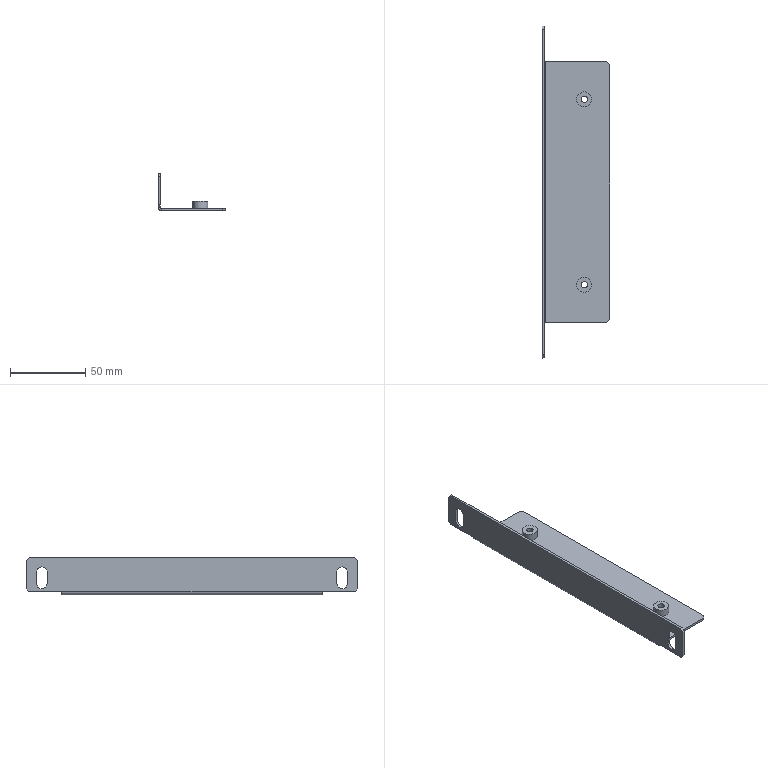Part | SolidWorks | features ICE 3, HoleWzd 2, Chamfer 1, FlatPattern 1, SMBaseFlange 1, SheetMetal 1 | 3 solids | 48 faces | box 45 x 220 x 25 mm | volume 19511 mm3 | plane 28 | cylinder 20 | commonest cylinder face diameters 7 x6 4.2 x4 5.5 x4 10 x4 1.473 x1 4.473 x1
STEP:
#1=CARTESIAN_POINT('',(25.9,61.5,-18.5));
#2=VERTEX_POINT('',#1);
#3=CARTESIAN_POINT('',(30.1,61.5,-18.5));
#4=VERTEX_POINT('',#3);
#5=CARTESIAN_POINT('',(28.,61.5,-18.5));
#6=DIRECTION('',(0.,0.,1.));
#7=DIRECTION('',(1.,0.,0.));
#8=AXIS2_PLACEMENT_3D('',#5,#6,#7);
#9=CIRCLE('',#8,2.1);
#10=EDGE_CURVE('',#2,#4,#9,.T.);
#11=ORIENTED_EDGE('',*,*,#10,.T.);
#12=CARTESIAN_POINT('',(30.1,61.5,-23.5));
#13=VERTEX_POINT('',#12);
#14=CARTESIAN_POINT('',(30.1,61.5,-23.5));
#15=DIRECTION('',(0.,0.,-1.));
#16=VECTOR('',#15,1000.);
#17=LINE('',#14,#16);
#18=EDGE_CURVE('',#4,#13,#17,.T.);
#19=ORIENTED_EDGE('',*,*,#18,.T.);
#20=CARTESIAN_POINT('',(25.9,61.5,-23.5));
#21=VERTEX_POINT('',#20);
#22=CARTESIAN_POINT('',(28.,61.5,-23.5));
#23=DIRECTION('',(0.,0.,-1.));
#24=DIRECTION('',(-1.,0.,0.));
#25=AXIS2_PLACEMENT_3D('',#22,#23,#24);
#26=CIRCLE('',#25,2.1);
#27=EDGE_CURVE('',#13,#21,#26,.T.);
#28=ORIENTED_EDGE('',*,*,#27,.T.);
#29=CARTESIAN_POINT('',(25.9,61.5,-23.5));
#30=DIRECTION('',(0.,0.,-1.));
#31=VECTOR('',#30,1000.);
#32=LINE('',#29,#31);
#33=EDGE_CURVE('',#2,#21,#32,.T.);
#34=ORIENTED_EDGE('',*,*,#33,.F.);
#35=EDGE_LOOP('',(#11,#19,#28,#34));
#36=FACE_OUTER_BOUND('',#35,.T.);
#37=CARTESIAN_POINT('',(28.,61.5,-23.5));
#38=DIRECTION('',(0.,0.,-1.));
#39=DIRECTION('',(-1.,0.,0.));
#40=AXIS2_PLACEMENT_3D('',#37,#38,#39);
#41=CYLINDRICAL_SURFACE('',#40,2.1);
#42=ADVANCED_FACE('',(#36),#41,.F.);
#43=CARTESIAN_POINT('',(33.,61.5,-18.5));
#44=VERTEX_POINT('',#43);
#45=CARTESIAN_POINT('',(23.,61.5,-18.5));
#46=VERTEX_POINT('',#45);
#47=CARTESIAN_POINT('',(28.,61.5,-18.5));
#48=DIRECTION('',(0.,0.,1.));
#49=DIRECTION('',(1.,0.,0.));
#50=AXIS2_PLACEMENT_3D('',#47,#48,#49);
#51=CIRCLE('',#50,5.);
#52=EDGE_CURVE('',#44,#46,#51,.T.);
#53=ORIENTED_EDGE('',*,*,#52,.F.);
#54=CARTESIAN_POINT('',(33.,61.5,-23.5));
#55=VERTEX_POINT('',#54);
#56=CARTESIAN_POINT('',(33.,61.5,-18.5));
#57=DIRECTION('',(0.,0.,-1.));
#58=VECTOR('',#57,1000.);
#59=LINE('',#56,#58);
#60=EDGE_CURVE('',#44,#55,#59,.T.);
#61=ORIENTED_EDGE('',*,*,#60,.T.);
#62=CARTESIAN_POINT('',(23.,61.5,-23.5));
#63=VERTEX_POINT('',#62);
#64=CARTESIAN_POINT('',(28.,61.5,-23.5));
#65=DIRECTION('',(0.,0.,1.));
#66=DIRECTION('',(1.,0.,0.));
#67=AXIS2_PLACEMENT_3D('',#64,#65,#66);
#68=CIRCLE('',#67,5.);
#69=EDGE_CURVE('',#55,#63,#68,.T.);
#70=ORIENTED_EDGE('',*,*,#69,.T.);
#71=CARTESIAN_POINT('',(23.,61.5,-18.5));
#72=DIRECTION('',(0.,0.,-1.));
#73=VECTOR('',#72,1000.);
#74=LINE('',#71,#73);
#75=EDGE_CURVE('',#46,#63,#74,.T.);
#76=ORIENTED_EDGE('',*,*,#75,.F.);
#77=EDGE_LOOP('',(#53,#61,#70,#76));
#78=FACE_OUTER_BOUND('',#77,.T.);
#79=CARTESIAN_POINT('',(28.,61.5,-18.5));
#80=DIRECTION('',(0.,0.,-1.));
#81=DIRECTION('',(-1.,0.,0.));
#82=AXIS2_PLACEMENT_3D('',#79,#80,#81);
#83=CYLINDRICAL_SURFACE('',#82,5.);
#84=ADVANCED_FACE('',(#78),#83,.T.);
#85=ORIENTED_EDGE('',*,*,#60,.F.);
#86=CARTESIAN_POINT('',(28.,61.5,-18.5));
#87=DIRECTION('',(0.,0.,1.));
#88=DIRECTION('',(1.,0.,0.));
#89=AXIS2_PLACEMENT_3D('',#86,#87,#88);
#90=CIRCLE('',#89,5.);
#91=EDGE_CURVE('',#46,#44,#90,.T.);
#92=ORIENTED_EDGE('',*,*,#91,.F.);
#93=ORIENTED_EDGE('',*,*,#75,.T.);
#94=CARTESIAN_POINT('',(28.,61.5,-23.5));
#95=DIRECTION('',(0.,0.,1.));
#96=DIRECTION('',(1.,0.,0.));
#97=AXIS2_PLACEMENT_3D('',#94,#95,#96);
#98=CIRCLE('',#97,5.);
#99=EDGE_CURVE('',#63,#55,#98,.T.);
#100=ORIENTED_EDGE('',*,*,#99,.T.);
#101=EDGE_LOOP('',(#85,#92,#93,#100));
#102=FACE_OUTER_BOUND('',#101,.T.);
#103=CARTESIAN_POINT('',(28.,61.5,-18.5));
#104=DIRECTION('',(0.,0.,-1.));
#105=DIRECTION('',(-1.,0.,0.));
#106=AXIS2_PLACEMENT_3D('',#103,#104,#105);
#107=CYLINDRICAL_SURFACE('',#106,5.);
#108=ADVANCED_FACE('',(#102),#107,.T.);
#109=ORIENTED_EDGE('',*,*,#10,.F.);
#110=CARTESIAN_POINT('',(28.,61.5,-18.5));
#111=DIRECTION('',(0.,0.,1.));
#112=DIRECTION('',(1.,0.,0.));
#113=AXIS2_PLACEMENT_3D('',#110,#111,#112);
#114=CIRCLE('',#113,2.1);
#115=EDGE_CURVE('',#4,#2,#114,.T.);
#116=ORIENTED_EDGE('',*,*,#115,.F.);
#117=EDGE_LOOP('',(#109,#116));
#118=FACE_BOUND('',#117,.T.);
#119=ORIENTED_EDGE('',*,*,#91,.T.);
#120=ORIENTED_EDGE('',*,*,#52,.T.);
#121=EDGE_LOOP('',(#119,#120));
#122=FACE_OUTER_BOUND('',#121,.T.);
#123=CARTESIAN_POINT('',(28.,61.5,-18.5));
#124=DIRECTION('',(0.,0.,1.));
#125=DIRECTION('',(1.,0.,0.));
#126=AXIS2_PLACEMENT_3D('',#123,#124,#125);
#127=PLANE('',#126);
#128=ADVANCED_FACE('',(#118,#122),#127,.T.);
#129=CARTESIAN_POINT('',(28.,61.5,-23.5));
#130=DIRECTION('',(0.,0.,-1.));
#131=DIRECTION('',(-1.,0.,0.));
#132=AXIS2_PLACEMENT_3D('',#129,#130,#131);
#133=CIRCLE('',#132,2.1);
#134=EDGE_CURVE('',#21,#13,#133,.T.);
#135=ORIENTED_EDGE('',*,*,#134,.F.);
#136=ORIENTED_EDGE('',*,*,#27,.F.);
#137=EDGE_LOOP('',(#135,#136));
#138=FACE_BOUND('',#137,.T.);
#139=ORIENTED_EDGE('',*,*,#99,.F.);
#140=ORIENTED_EDGE('',*,*,#69,.F.);
#141=EDGE_LOOP('',(#139,#140));
#142=FACE_OUTER_BOUND('',#141,.T.);
#143=CARTESIAN_POINT('',(28.,61.5,-23.5));
#144=DIRECTION('',(0.,0.,1.));
#145=DIRECTION('',(1.,0.,0.));
#146=AXIS2_PLACEMENT_3D('',#143,#144,#145);
#147=PLANE('',#146);
#148=ADVANCED_FACE('',(#138,#142),#147,.F.);
#149=ORIENTED_EDGE('',*,*,#18,.F.);
#150=ORIENTED_EDGE('',*,*,#115,.T.);
#151=ORIENTED_EDGE('',*,*,#33,.T.);
#152=ORIENTED_EDGE('',*,*,#134,.T.);
#153=EDGE_LOOP('',(#149,#150,#151,#152));
#154=FACE_OUTER_BOUND('',#153,.T.);
#155=CARTESIAN_POINT('',(28.,61.5,-23.5));
#156=DIRECTION('',(0.,0.,-1.));
#157=DIRECTION('',(-1.,0.,0.));
#158=AXIS2_PLACEMENT_3D('',#155,#156,#157);
#159=CYLINDRICAL_SURFACE('',#158,2.1);
#160=ADVANCED_FACE('',(#154),#159,.F.);
#161=CLOSED_SHELL('',(#42,#84,#108,#128,#148,#160));
#162=MANIFOLD_SOLID_BREP('',#161);
#163=CARTESIAN_POINT('',(25.9,-61.5,-18.5));
#164=VERTEX_POINT('',#163);
#165=CARTESIAN_POINT('',(30.1,-61.5,-18.5));
#166=VERTEX_POINT('',#165);
#167=CARTESIAN_POINT('',(28.,-61.5,-18.5));
#168=DIRECTION('',(0.,0.,1.));
#169=DIRECTION('',(1.,0.,0.));
#170=AXIS2_PLACEMENT_3D('',#167,#168,#169);
#171=CIRCLE('',#170,2.1);
#172=EDGE_CURVE('',#164,#166,#171,.T.);
#173=ORIENTED_EDGE('',*,*,#172,.T.);
#174=CARTESIAN_POINT('',(30.1,-61.5,-23.5));
#175=VERTEX_POINT('',#174);
#176=CARTESIAN_POINT('',(30.1,-61.5,-23.5));
#177=DIRECTION('',(0.,0.,-1.));
#178=VECTOR('',#177,1000.);
#179=LINE('',#176,#178);
#180=EDGE_CURVE('',#166,#175,#179,.T.);
#181=ORIENTED_EDGE('',*,*,#180,.T.);
#182=CARTESIAN_POINT('',(25.9,-61.5,-23.5));
#183=VERTEX_POINT('',#182);
#184=CARTESIAN_POINT('',(28.,-61.5,-23.5));
#185=DIRECTION('',(0.,0.,-1.));
#186=DIRECTION('',(-1.,0.,0.));
#187=AXIS2_PLACEMENT_3D('',#184,#185,#186);
#188=CIRCLE('',#187,2.1);
#189=EDGE_CURVE('',#175,#183,#188,.T.);
#190=ORIENTED_EDGE('',*,*,#189,.T.);
#191=CARTESIAN_POINT('',(25.9,-61.5,-23.5));
#192=DIRECTION('',(0.,0.,-1.));
#193=VECTOR('',#192,1000.);
#194=LINE('',#191,#193);
#195=EDGE_CURVE('',#164,#183,#194,.T.);
#196=ORIENTED_EDGE('',*,*,#195,.F.);
#197=EDGE_LOOP('',(#173,#181,#190,#196));
#198=FACE_OUTER_BOUND('',#197,.T.);
#199=CARTESIAN_POINT('',(28.,-61.5,-23.5));
#200=DIRECTION('',(0.,0.,-1.));
#201=DIRECTION('',(-1.,0.,0.));
#202=AXIS2_PLACEMENT_3D('',#199,#200,#201);
#203=CYLINDRICAL_SURFACE('',#202,2.1);
#204=ADVANCED_FACE('',(#198),#203,.F.);
#205=CARTESIAN_POINT('',(33.,-61.5,-18.5));
#206=VERTEX_POINT('',#205);
#207=CARTESIAN_POINT('',(23.,-61.5,-18.5));
#208=VERTEX_POINT('',#207);
#209=CARTESIAN_POINT('',(28.,-61.5,-18.5));
#210=DIRECTION('',(0.,0.,1.));
#211=DIRECTION('',(1.,0.,0.));
#212=AXIS2_PLACEMENT_3D('',#209,#210,#211);
#213=CIRCLE('',#212,5.);
#214=EDGE_CURVE('',#206,#208,#213,.T.);
#215=ORIENTED_EDGE('',*,*,#214,.F.);
#216=CARTESIAN_POINT('',(33.,-61.5,-23.5));
#217=VERTEX_POINT('',#216);
#218=CARTESIAN_POINT('',(33.,-61.5,-18.5));
#219=DIRECTION('',(0.,0.,-1.));
#220=VECTOR('',#219,1000.);
#221=LINE('',#218,#220);
#222=EDGE_CURVE('',#206,#217,#221,.T.);
#223=ORIENTED_EDGE('',*,*,#222,.T.);
#224=CARTESIAN_POINT('',(23.,-61.5,-23.5));
#225=VERTEX_POINT('',#224);
#226=CARTESIAN_POINT('',(28.,-61.5,-23.5));
#227=DIRECTION('',(0.,0.,1.));
#228=DIRECTION('',(1.,0.,0.));
#229=AXIS2_PLACEMENT_3D('',#226,#227,#228);
#230=CIRCLE('',#229,5.);
#231=EDGE_CURVE('',#217,#225,#230,.T.);
#232=ORIENTED_EDGE('',*,*,#231,.T.);
#233=CARTESIAN_POINT('',(23.,-61.5,-18.5));
#234=DIRECTION('',(0.,0.,-1.));
#235=VECTOR('',#234,1000.);
#236=LINE('',#233,#235);
#237=EDGE_CURVE('',#208,#225,#236,.T.);
#238=ORIENTED_EDGE('',*,*,#237,.F.);
#239=EDGE_LOOP('',(#215,#223,#232,#238));
#240=FACE_OUTER_BOUND('',#239,.T.);
#241=CARTESIAN_POINT('',(28.,-61.5,-18.5));
#242=DIRECTION('',(0.,0.,-1.));
#243=DIRECTION('',(-1.,0.,0.));
#244=AXIS2_PLACEMENT_3D('',#241,#242,#243);
#245=CYLINDRICAL_SURFACE('',#244,5.);
#246=ADVANCED_FACE('',(#240),#245,.T.);
#247=ORIENTED_EDGE('',*,*,#222,.F.);
#248=CARTESIAN_POINT('',(28.,-61.5,-18.5));
#249=DIRECTION('',(0.,0.,1.));
#250=DIRECTION('',(1.,0.,0.));
#251=AXIS2_PLACEMENT_3D('',#248,#249,#250);
#252=CIRCLE('',#251,5.);
#253=EDGE_CURVE('',#208,#206,#252,.T.);
#254=ORIENTED_EDGE('',*,*,#253,.F.);
#255=ORIENTED_EDGE('',*,*,#237,.T.);
#256=CARTESIAN_POINT('',(28.,-61.5,-23.5));
#257=DIRECTION('',(0.,0.,1.));
#258=DIRECTION('',(1.,0.,0.));
#259=AXIS2_PLACEMENT_3D('',#256,#257,#258);
#260=CIRCLE('',#259,5.);
#261=EDGE_CURVE('',#225,#217,#260,.T.);
#262=ORIENTED_EDGE('',*,*,#261,.T.);
#263=EDGE_LOOP('',(#247,#254,#255,#262));
#264=FACE_OUTER_BOUND('',#263,.T.);
#265=CARTESIAN_POINT('',(28.,-61.5,-18.5));
#266=DIRECTION('',(0.,0.,-1.));
#267=DIRECTION('',(-1.,0.,0.));
#268=AXIS2_PLACEMENT_3D('',#265,#266,#267);
#269=CYLINDRICAL_SURFACE('',#268,5.);
#270=ADVANCED_FACE('',(#264),#269,.T.);
#271=ORIENTED_EDGE('',*,*,#172,.F.);
#272=CARTESIAN_POINT('',(28.,-61.5,-18.5));
#273=DIRECTION('',(0.,0.,1.));
#274=DIRECTION('',(1.,0.,0.));
#275=AXIS2_PLACEMENT_3D('',#272,#273,#274);
#276=CIRCLE('',#275,2.1);
#277=EDGE_CURVE('',#166,#164,#276,.T.);
#278=ORIENTED_EDGE('',*,*,#277,.F.);
#279=EDGE_LOOP('',(#271,#278));
#280=FACE_BOUND('',#279,.T.);
#281=ORIENTED_EDGE('',*,*,#253,.T.);
#282=ORIENTED_EDGE('',*,*,#214,.T.);
#283=EDGE_LOOP('',(#281,#282));
#284=FACE_OUTER_BOUND('',#283,.T.);
#285=CARTESIAN_POINT('',(28.,-61.5,-18.5));
#286=DIRECTION('',(0.,0.,1.));
#287=DIRECTION('',(1.,0.,0.));
#288=AXIS2_PLACEMENT_3D('',#285,#286,#287);
#289=PLANE('',#288);
#290=ADVANCED_FACE('',(#280,#284),#289,.T.);
#291=CARTESIAN_POINT('',(28.,-61.5,-23.5));
#292=DIRECTION('',(0.,0.,-1.));
#293=DIRECTION('',(-1.,0.,0.));
#294=AXIS2_PLACEMENT_3D('',#291,#292,#293);
#295=CIRCLE('',#294,2.1);
#296=EDGE_CURVE('',#183,#175,#295,.T.);
#297=ORIENTED_EDGE('',*,*,#296,.F.);
#298=ORIENTED_EDGE('',*,*,#189,.F.);
#299=EDGE_LOOP('',(#297,#298));
#300=FACE_BOUND('',#299,.T.);
#301=ORIENTED_EDGE('',*,*,#261,.F.);
#302=ORIENTED_EDGE('',*,*,#231,.F.);
#303=EDGE_LOOP('',(#301,#302));
#304=FACE_OUTER_BOUND('',#303,.T.);
#305=CARTESIAN_POINT('',(28.,-61.5,-23.5));
#306=DIRECTION('',(0.,0.,1.));
#307=DIRECTION('',(1.,0.,0.));
#308=AXIS2_PLACEMENT_3D('',#305,#306,#307);
#309=PLANE('',#308);
#310=ADVANCED_FACE('',(#300,#304),#309,.F.);
#311=ORIENTED_EDGE('',*,*,#180,.F.);
#312=ORIENTED_EDGE('',*,*,#277,.T.);
#313=ORIENTED_EDGE('',*,*,#195,.T.);
#314=ORIENTED_EDGE('',*,*,#296,.T.);
#315=EDGE_LOOP('',(#311,#312,#313,#314));
#316=FACE_OUTER_BOUND('',#315,.T.);
#317=CARTESIAN_POINT('',(28.,-61.5,-23.5));
#318=DIRECTION('',(0.,0.,-1.));
#319=DIRECTION('',(-1.,0.,0.));
#320=AXIS2_PLACEMENT_3D('',#317,#318,#319);
#321=CYLINDRICAL_SURFACE('',#320,2.1);
#322=ADVANCED_FACE('',(#316),#321,.F.);
#323=CLOSED_SHELL('',(#204,#246,#270,#290,#310,#322));
#324=MANIFOLD_SOLID_BREP('',#323);
#325=CARTESIAN_POINT('',(1.5,-99.5,-6.5));
#326=VERTEX_POINT('',#325);
#327=CARTESIAN_POINT('',(1.5,-96.,-10.));
#328=VERTEX_POINT('',#327);
#329=CARTESIAN_POINT('',(1.5,-99.5,-10.));
#330=DIRECTION('',(-1.,0.,0.));
#331=DIRECTION('',(0.,0.,1.));
#332=AXIS2_PLACEMENT_3D('',#329,#330,#331);
#333=CIRCLE('',#332,3.5);
#334=EDGE_CURVE('',#326,#328,#333,.T.);
#335=ORIENTED_EDGE('',*,*,#334,.F.);
#336=CARTESIAN_POINT('',(0.,-99.5,-6.5));
#337=VERTEX_POINT('',#336);
#338=CARTESIAN_POINT('',(5.,-99.5,-6.5));
#339=DIRECTION('',(-1.,0.,0.));
#340=VECTOR('',#339,1000.);
#341=LINE('',#338,#340);
#342=EDGE_CURVE('',#326,#337,#341,.T.);
#343=ORIENTED_EDGE('',*,*,#342,.T.);
#344=CARTESIAN_POINT('',(0.,-96.,-10.));
#345=VERTEX_POINT('',#344);
#346=CARTESIAN_POINT('',(0.,-99.5,-10.));
#347=DIRECTION('',(-1.,0.,0.));
#348=DIRECTION('',(0.,0.,1.));
#349=AXIS2_PLACEMENT_3D('',#346,#347,#348);
#350=CIRCLE('',#349,3.5);
#351=EDGE_CURVE('',#337,#345,#350,.T.);
#352=ORIENTED_EDGE('',*,*,#351,.T.);
#353=CARTESIAN_POINT('',(5.,-96.,-10.));
#354=DIRECTION('',(-1.,0.,0.));
#355=VECTOR('',#354,1000.);
#356=LINE('',#353,#355);
#357=EDGE_CURVE('',#328,#345,#356,.T.);
#358=ORIENTED_EDGE('',*,*,#357,.F.);
#359=EDGE_LOOP('',(#335,#343,#352,#358));
#360=FACE_OUTER_BOUND('',#359,.T.);
#361=CARTESIAN_POINT('',(5.,-99.5,-10.));
#362=DIRECTION('',(-1.,0.,0.));
#363=DIRECTION('',(0.,0.,1.));
#364=AXIS2_PLACEMENT_3D('',#361,#362,#363);
#365=CYLINDRICAL_SURFACE('',#364,3.5);
#366=ADVANCED_FACE('',(#360),#365,.F.);
#367=CARTESIAN_POINT('',(1.5,99.5,-6.5));
#368=VERTEX_POINT('',#367);
#369=CARTESIAN_POINT('',(1.5,103.,-10.));
#370=VERTEX_POINT('',#369);
#371=CARTESIAN_POINT('',(1.5,99.5,-10.));
#372=DIRECTION('',(-1.,0.,0.));
#373=DIRECTION('',(0.,0.,1.));
#374=AXIS2_PLACEMENT_3D('',#371,#372,#373);
#375=CIRCLE('',#374,3.5);
#376=EDGE_CURVE('',#368,#370,#375,.T.);
#377=ORIENTED_EDGE('',*,*,#376,.F.);
#378=CARTESIAN_POINT('',(0.,99.5,-6.5));
#379=VERTEX_POINT('',#378);
#380=CARTESIAN_POINT('',(5.,99.5,-6.5));
#381=DIRECTION('',(-1.,0.,0.));
#382=VECTOR('',#381,1000.);
#383=LINE('',#380,#382);
#384=EDGE_CURVE('',#368,#379,#383,.T.);
#385=ORIENTED_EDGE('',*,*,#384,.T.);
#386=CARTESIAN_POINT('',(0.,103.,-10.));
#387=VERTEX_POINT('',#386);
#388=CARTESIAN_POINT('',(0.,99.5,-10.));
#389=DIRECTION('',(-1.,0.,0.));
#390=DIRECTION('',(0.,0.,1.));
#391=AXIS2_PLACEMENT_3D('',#388,#389,#390);
#392=CIRCLE('',#391,3.5);
#393=EDGE_CURVE('',#379,#387,#392,.T.);
#394=ORIENTED_EDGE('',*,*,#393,.T.);
#395=CARTESIAN_POINT('',(5.,103.,-10.));
#396=DIRECTION('',(-1.,0.,0.));
#397=VECTOR('',#396,1000.);
#398=LINE('',#395,#397);
#399=EDGE_CURVE('',#370,#387,#398,.T.);
#400=ORIENTED_EDGE('',*,*,#399,.F.);
#401=EDGE_LOOP('',(#377,#385,#394,#400));
#402=FACE_OUTER_BOUND('',#401,.T.);
#403=CARTESIAN_POINT('',(5.,99.5,-10.));
#404=DIRECTION('',(-1.,0.,0.));
#405=DIRECTION('',(0.,0.,1.));
#406=AXIS2_PLACEMENT_3D('',#403,#404,#405);
#407=CYLINDRICAL_SURFACE('',#406,3.5);
#408=ADVANCED_FACE('',(#402),#407,.F.);
#409=CARTESIAN_POINT('',(30.75,61.5,-23.5));
#410=VERTEX_POINT('',#409);
#411=CARTESIAN_POINT('',(25.25,61.5,-23.5));
#412=VERTEX_POINT('',#411);
#413=CARTESIAN_POINT('',(28.,61.5,-23.5));
#414=DIRECTION('',(0.,0.,-1.));
#415=DIRECTION('',(-1.,0.,0.));
#416=AXIS2_PLACEMENT_3D('',#413,#414,#415);
#417=CIRCLE('',#416,2.75);
#418=EDGE_CURVE('',#410,#412,#417,.T.);
#419=ORIENTED_EDGE('',*,*,#418,.F.);
#420=CARTESIAN_POINT('',(30.75,61.5,-25.));
#421=VERTEX_POINT('',#420);
#422=CARTESIAN_POINT('',(30.75,61.5,-25.));
#423=DIRECTION('',(0.,0.,-1.));
#424=VECTOR('',#423,1000.);
#425=LINE('',#422,#424);
#426=EDGE_CURVE('',#410,#421,#425,.T.);
#427=ORIENTED_EDGE('',*,*,#426,.T.);
#428=CARTESIAN_POINT('',(25.25,61.5,-25.));
#429=VERTEX_POINT('',#428);
#430=CARTESIAN_POINT('',(28.,61.5,-25.));
#431=DIRECTION('',(0.,0.,-1.));
#432=DIRECTION('',(-1.,0.,0.));
#433=AXIS2_PLACEMENT_3D('',#430,#431,#432);
#434=CIRCLE('',#433,2.75);
#435=EDGE_CURVE('',#421,#429,#434,.T.);
#436=ORIENTED_EDGE('',*,*,#435,.T.);
#437=CARTESIAN_POINT('',(25.25,61.5,-25.));
#438=DIRECTION('',(0.,0.,-1.));
#439=VECTOR('',#438,1000.);
#440=LINE('',#437,#439);
#441=EDGE_CURVE('',#412,#429,#440,.T.);
#442=ORIENTED_EDGE('',*,*,#441,.F.);
#443=EDGE_LOOP('',(#419,#427,#436,#442));
#444=FACE_OUTER_BOUND('',#443,.T.);
#445=CARTESIAN_POINT('',(28.,61.5,-25.));
#446=DIRECTION('',(0.,0.,-1.));
#447=DIRECTION('',(-1.,0.,0.));
#448=AXIS2_PLACEMENT_3D('',#445,#446,#447);
#449=CYLINDRICAL_SURFACE('',#448,2.75);
#450=ADVANCED_FACE('',(#444),#449,.F.);
#451=CARTESIAN_POINT('',(30.75,-61.5,-23.5));
#452=VERTEX_POINT('',#451);
#453=CARTESIAN_POINT('',(25.25,-61.5,-23.5));
#454=VERTEX_POINT('',#453);
#455=CARTESIAN_POINT('',(28.,-61.5,-23.5));
#456=DIRECTION('',(0.,0.,-1.));
#457=DIRECTION('',(-1.,0.,0.));
#458=AXIS2_PLACEMENT_3D('',#455,#456,#457);
#459=CIRCLE('',#458,2.75);
#460=EDGE_CURVE('',#452,#454,#459,.T.);
#461=ORIENTED_EDGE('',*,*,#460,.F.);
#462=CARTESIAN_POINT('',(30.75,-61.5,-25.));
#463=VERTEX_POINT('',#462);
#464=CARTESIAN_POINT('',(30.75,-61.5,-25.));
#465=DIRECTION('',(0.,0.,-1.));
#466=VECTOR('',#465,1000.);
#467=LINE('',#464,#466);
#468=EDGE_CURVE('',#452,#463,#467,.T.);
#469=ORIENTED_EDGE('',*,*,#468,.T.);
#470=CARTESIAN_POINT('',(25.25,-61.5,-25.));
#471=VERTEX_POINT('',#470);
#472=CARTESIAN_POINT('',(28.,-61.5,-25.));
#473=DIRECTION('',(0.,0.,-1.));
#474=DIRECTION('',(-1.,0.,0.));
#475=AXIS2_PLACEMENT_3D('',#472,#473,#474);
#476=CIRCLE('',#475,2.75);
#477=EDGE_CURVE('',#463,#471,#476,.T.);
#478=ORIENTED_EDGE('',*,*,#477,.T.);
#479=CARTESIAN_POINT('',(25.25,-61.5,-25.));
#480=DIRECTION('',(0.,0.,-1.));
#481=VECTOR('',#480,1000.);
#482=LINE('',#479,#481);
#483=EDGE_CURVE('',#454,#471,#482,.T.);
#484=ORIENTED_EDGE('',*,*,#483,.F.);
#485=EDGE_LOOP('',(#461,#469,#478,#484));
#486=FACE_OUTER_BOUND('',#485,.T.);
#487=CARTESIAN_POINT('',(28.,-61.5,-25.));
#488=DIRECTION('',(0.,0.,-1.));
#489=DIRECTION('',(-1.,0.,0.));
#490=AXIS2_PLACEMENT_3D('',#487,#488,#489);
#491=CYLINDRICAL_SURFACE('',#490,2.75);
#492=ADVANCED_FACE('',(#486),#491,.F.);
#493=CARTESIAN_POINT('',(28.,61.5,-23.5));
#494=DIRECTION('',(0.,0.,-1.));
#495=DIRECTION('',(-1.,0.,0.));
#496=AXIS2_PLACEMENT_3D('',#493,#494,#495);
#497=CIRCLE('',#496,2.75);
#498=EDGE_CURVE('',#412,#410,#497,.T.);
#499=ORIENTED_EDGE('',*,*,#498,.T.);
#500=ORIENTED_EDGE('',*,*,#418,.T.);
#501=EDGE_LOOP('',(#499,#500));
#502=FACE_BOUND('',#501,.T.);
#503=CARTESIAN_POINT('',(28.,-61.5,-23.5));
#504=DIRECTION('',(0.,0.,-1.));
#505=DIRECTION('',(-1.,0.,0.));
#506=AXIS2_PLACEMENT_3D('',#503,#504,#505);
#507=CIRCLE('',#506,2.75);
#508=EDGE_CURVE('',#454,#452,#507,.T.);
#509=ORIENTED_EDGE('',*,*,#508,.T.);
#510=ORIENTED_EDGE('',*,*,#460,.T.);
#511=EDGE_LOOP('',(#509,#510));
#512=FACE_BOUND('',#511,.T.);
#513=CARTESIAN_POINT('',(2.237,-86.5,-23.5));
#514=VERTEX_POINT('',#513);
#515=CARTESIAN_POINT('',(43.,-86.5,-23.5));
#516=VERTEX_POINT('',#515);
#517=CARTESIAN_POINT('',(0.,-86.5,-23.5));
#518=DIRECTION('',(1.,0.,0.));
#519=VECTOR('',#518,1000.);
#520=LINE('',#517,#519);
#521=EDGE_CURVE('',#514,#516,#520,.T.);
#522=ORIENTED_EDGE('',*,*,#521,.T.);
#523=CARTESIAN_POINT('',(45.,-84.5,-23.5));
#524=VERTEX_POINT('',#523);
#525=CARTESIAN_POINT('',(45.,-84.5,-23.5));
#526=DIRECTION('',(0.7071,0.7071,0.));
#527=VECTOR('',#526,1000.);
#528=LINE('',#525,#527);
#529=EDGE_CURVE('',#516,#524,#528,.T.);
#530=ORIENTED_EDGE('',*,*,#529,.T.);
#531=CARTESIAN_POINT('',(45.,84.5,-23.5));
#532=VERTEX_POINT('',#531);
#533=CARTESIAN_POINT('',(45.,110.,-23.5));
#534=DIRECTION('',(0.,-1.,0.));
#535=VECTOR('',#534,1000.);
#536=LINE('',#533,#535);
#537=EDGE_CURVE('',#532,#524,#536,.T.);
#538=ORIENTED_EDGE('',*,*,#537,.F.);
#539=CARTESIAN_POINT('',(43.,86.5,-23.5));
#540=VERTEX_POINT('',#539);
#541=CARTESIAN_POINT('',(45.,84.5,-23.5));
#542=DIRECTION('',(-0.7071,0.7071,0.));
#543=VECTOR('',#542,1000.);
#544=LINE('',#541,#543);
#545=EDGE_CURVE('',#532,#540,#544,.T.);
#546=ORIENTED_EDGE('',*,*,#545,.T.);
#547=CARTESIAN_POINT('',(2.237,86.5,-23.5));
#548=VERTEX_POINT('',#547);
#549=CARTESIAN_POINT('',(0.,86.5,-23.5));
#550=DIRECTION('',(-1.,0.,0.));
#551=VECTOR('',#550,1000.);
#552=LINE('',#549,#551);
#553=EDGE_CURVE('',#540,#548,#552,.T.);
#554=ORIENTED_EDGE('',*,*,#553,.T.);
#555=CARTESIAN_POINT('',(2.237,110.,-23.5));
#556=DIRECTION('',(0.,-1.,0.));
#557=VECTOR('',#556,1000.);
#558=LINE('',#555,#557);
#559=EDGE_CURVE('',#548,#514,#558,.T.);
#560=ORIENTED_EDGE('',*,*,#559,.T.);
#561=EDGE_LOOP('',(#522,#530,#538,#546,#554,#560));
#562=FACE_OUTER_BOUND('',#561,.T.);
#563=CARTESIAN_POINT('',(0.,110.,-23.5));
#564=DIRECTION('',(0.,0.,-1.));
#565=DIRECTION('',(-1.,0.,0.));
#566=AXIS2_PLACEMENT_3D('',#563,#564,#565);
#567=PLANE('',#566);
#568=ADVANCED_FACE('',(#502,#512,#562),#567,.F.);
#569=ORIENTED_EDGE('',*,*,#537,.T.);
#570=CARTESIAN_POINT('',(45.,-84.5,-25.));
#571=VERTEX_POINT('',#570);
#572=CARTESIAN_POINT('',(45.,-84.5,-25.));
#573=DIRECTION('',(0.,0.,-1.));
#574=VECTOR('',#573,1000.);
#575=LINE('',#572,#574);
#576=EDGE_CURVE('',#524,#571,#575,.T.);
#577=ORIENTED_EDGE('',*,*,#576,.T.);
#578=CARTESIAN_POINT('',(45.,84.5,-25.));
#579=VERTEX_POINT('',#578);
#580=CARTESIAN_POINT('',(45.,110.,-25.));
#581=DIRECTION('',(0.,-1.,0.));
#582=VECTOR('',#581,1000.);
#583=LINE('',#580,#582);
#584=EDGE_CURVE('',#579,#571,#583,.T.);
#585=ORIENTED_EDGE('',*,*,#584,.F.);
#586=CARTESIAN_POINT('',(45.,84.5,-25.));
#587=DIRECTION('',(0.,0.,1.));
#588=VECTOR('',#587,1000.);
#589=LINE('',#586,#588);
#590=EDGE_CURVE('',#579,#532,#589,.T.);
#591=ORIENTED_EDGE('',*,*,#590,.T.);
#592=EDGE_LOOP('',(#569,#577,#585,#591));
#593=FACE_OUTER_BOUND('',#592,.T.);
#594=CARTESIAN_POINT('',(45.,110.,-25.));
#595=DIRECTION('',(1.,0.,0.));
#596=DIRECTION('',(0.,0.,-1.));
#597=AXIS2_PLACEMENT_3D('',#594,#595,#596);
#598=PLANE('',#597);
#599=ADVANCED_FACE('',(#593),#598,.T.);
#600=CARTESIAN_POINT('',(28.,61.5,-25.));
#601=DIRECTION('',(0.,0.,-1.));
#602=DIRECTION('',(-1.,0.,0.));
#603=AXIS2_PLACEMENT_3D('',#600,#601,#602);
#604=CIRCLE('',#603,2.75);
#605=EDGE_CURVE('',#429,#421,#604,.T.);
#606=ORIENTED_EDGE('',*,*,#605,.F.);
#607=ORIENTED_EDGE('',*,*,#435,.F.);
#608=EDGE_LOOP('',(#606,#607));
#609=FACE_BOUND('',#608,.T.);
#610=CARTESIAN_POINT('',(28.,-61.5,-25.));
#611=DIRECTION('',(0.,0.,-1.));
#612=DIRECTION('',(-1.,0.,0.));
#613=AXIS2_PLACEMENT_3D('',#610,#611,#612);
#614=CIRCLE('',#613,2.75);
#615=EDGE_CURVE('',#471,#463,#614,.T.);
#616=ORIENTED_EDGE('',*,*,#615,.F.);
#617=ORIENTED_EDGE('',*,*,#477,.F.);
#618=EDGE_LOOP('',(#616,#617));
#619=FACE_BOUND('',#618,.T.);
#620=ORIENTED_EDGE('',*,*,#584,.T.);
#621=CARTESIAN_POINT('',(43.,-86.5,-25.));
#622=VERTEX_POINT('',#621);
#623=CARTESIAN_POINT('',(119.75,-9.75,-25.));
#624=DIRECTION('',(-0.7071,-0.7071,0.));
#625=VECTOR('',#624,1000.);
#626=LINE('',#623,#625);
#627=EDGE_CURVE('',#571,#622,#626,.T.);
#628=ORIENTED_EDGE('',*,*,#627,.T.);
#629=CARTESIAN_POINT('',(2.237,-86.5,-25.));
#630=VERTEX_POINT('',#629);
#631=CARTESIAN_POINT('',(0.,-86.5,-25.));
#632=DIRECTION('',(1.,0.,0.));
#633=VECTOR('',#632,1000.);
#634=LINE('',#631,#633);
#635=EDGE_CURVE('',#630,#622,#634,.T.);
#636=ORIENTED_EDGE('',*,*,#635,.F.);
#637=CARTESIAN_POINT('',(2.237,86.5,-25.));
#638=VERTEX_POINT('',#637);
#639=CARTESIAN_POINT('',(2.237,110.,-25.));
#640=DIRECTION('',(0.,-1.,0.));
#641=VECTOR('',#640,1000.);
#642=LINE('',#639,#641);
#643=EDGE_CURVE('',#638,#630,#642,.T.);
#644=ORIENTED_EDGE('',*,*,#643,.F.);
#645=CARTESIAN_POINT('',(43.,86.5,-25.));
#646=VERTEX_POINT('',#645);
#647=CARTESIAN_POINT('',(45.,86.5,-25.));
#648=DIRECTION('',(-1.,0.,0.));
#649=VECTOR('',#648,1000.);
#650=LINE('',#647,#649);
#651=EDGE_CURVE('',#646,#638,#650,.T.);
#652=ORIENTED_EDGE('',*,*,#651,.F.);
#653=CARTESIAN_POINT('',(9.75,119.75,-25.));
#654=DIRECTION('',(0.7071,-0.7071,0.));
#655=VECTOR('',#654,1000.);
#656=LINE('',#653,#655);
#657=EDGE_CURVE('',#646,#579,#656,.T.);
#658=ORIENTED_EDGE('',*,*,#657,.T.);
#659=EDGE_LOOP('',(#620,#628,#636,#644,#652,#658));
#660=FACE_OUTER_BOUND('',#659,.T.);
#661=CARTESIAN_POINT('',(0.,110.,-25.));
#662=DIRECTION('',(0.,0.,-1.));
#663=DIRECTION('',(-1.,0.,0.));
#664=AXIS2_PLACEMENT_3D('',#661,#662,#663);
#665=PLANE('',#664);
#666=ADVANCED_FACE('',(#609,#619,#660),#665,.T.);
#667=CARTESIAN_POINT('',(0.,108.237,-22.763));
#668=VERTEX_POINT('',#667);
#669=CARTESIAN_POINT('',(0.,-108.237,-22.763));
#670=VERTEX_POINT('',#669);
#671=CARTESIAN_POINT('',(0.,110.,-22.763));
#672=DIRECTION('',(0.,-1.,0.));
#673=VECTOR('',#672,1000.);
#674=LINE('',#671,#673);
#675=EDGE_CURVE('',#668,#670,#674,.T.);
#676=ORIENTED_EDGE('',*,*,#675,.F.);
#677=CARTESIAN_POINT('',(0.01255,108.,-23.));
#678=VERTEX_POINT('',#677);
#679=CARTESIAN_POINT('',(0.,108.237,-22.763));
#680=CARTESIAN_POINT('',(0.,108.158,-22.842));
#681=CARTESIAN_POINT('',(0.004187,108.079,-22.921));
#682=CARTESIAN_POINT('',(0.01255,108.,-23.));
#683=(BOUNDED_CURVE()B_SPLINE_CURVE(3,(#679,#680,#681,#682),.UNSPECIFIED.,.F.,.F.)B_SPLINE_CURVE_WITH_KNOTS((4,4),(4.606,4.712),.UNSPECIFIED.)CURVE()GEOMETRIC_REPRESENTATION_ITEM()RATIONAL_B_SPLINE_CURVE((1.,0.9991,0.9991,1.))REPRESENTATION_ITEM(''));
#684=EDGE_CURVE('',#668,#678,#683,.T.);
#685=ORIENTED_EDGE('',*,*,#684,.T.);
#686=CARTESIAN_POINT('',(0.01255,86.5,-23.));
#687=VERTEX_POINT('',#686);
#688=CARTESIAN_POINT('',(0.01255,110.,-23.));
#689=DIRECTION('',(0.,-1.,0.));
#690=VECTOR('',#689,1000.);
#691=LINE('',#688,#690);
#692=EDGE_CURVE('',#678,#687,#691,.T.);
#693=ORIENTED_EDGE('',*,*,#692,.T.);
#694=CARTESIAN_POINT('',(2.237,86.5,-22.763));
#695=DIRECTION('',(0.,1.,0.));
#696=DIRECTION('',(1.,0.,0.));
#697=AXIS2_PLACEMENT_3D('',#694,#695,#696);
#698=CIRCLE('',#697,2.237);
#699=EDGE_CURVE('',#638,#687,#698,.T.);
#700=ORIENTED_EDGE('',*,*,#699,.F.);
#701=ORIENTED_EDGE('',*,*,#643,.T.);
#702=CARTESIAN_POINT('',(0.01255,-86.5,-23.));
#703=VERTEX_POINT('',#702);
#704=CARTESIAN_POINT('',(2.237,-86.5,-22.763));
#705=DIRECTION('',(0.,-1.,0.));
#706=DIRECTION('',(-1.,0.,0.));
#707=AXIS2_PLACEMENT_3D('',#704,#705,#706);
#708=CIRCLE('',#707,2.237);
#709=EDGE_CURVE('',#703,#630,#708,.T.);
#710=ORIENTED_EDGE('',*,*,#709,.F.);
#711=CARTESIAN_POINT('',(0.01255,-108.,-23.));
#712=VERTEX_POINT('',#711);
#713=CARTESIAN_POINT('',(0.01255,110.,-23.));
#714=DIRECTION('',(0.,1.,0.));
#715=VECTOR('',#714,1000.);
#716=LINE('',#713,#715);
#717=EDGE_CURVE('',#712,#703,#716,.T.);
#718=ORIENTED_EDGE('',*,*,#717,.F.);
#719=CARTESIAN_POINT('',(0.01255,-108.,-23.));
#720=CARTESIAN_POINT('',(0.004187,-108.079,-22.921));
#721=CARTESIAN_POINT('',(0.,-108.158,-22.842));
#722=CARTESIAN_POINT('',(0.,-108.237,-22.763));
#723=(BOUNDED_CURVE()B_SPLINE_CURVE(3,(#719,#720,#721,#722),.UNSPECIFIED.,.F.,.F.)B_SPLINE_CURVE_WITH_KNOTS((4,4),(4.712,4.818),.UNSPECIFIED.)CURVE()GEOMETRIC_REPRESENTATION_ITEM()RATIONAL_B_SPLINE_CURVE((1.,0.9991,0.9991,1.))REPRESENTATION_ITEM(''));
#724=EDGE_CURVE('',#712,#670,#723,.T.);
#725=ORIENTED_EDGE('',*,*,#724,.T.);
#726=EDGE_LOOP('',(#676,#685,#693,#700,#701,#710,#718,#725));
#727=FACE_OUTER_BOUND('',#726,.T.);
#728=CARTESIAN_POINT('',(2.237,110.,-22.763));
#729=DIRECTION('',(0.,-1.,0.));
#730=DIRECTION('',(0.,0.,-1.));
#731=AXIS2_PLACEMENT_3D('',#728,#729,#730);
#732=CYLINDRICAL_SURFACE('',#731,2.237);
#733=ADVANCED_FACE('',(#727),#732,.T.);
#734=CARTESIAN_POINT('',(1.504,108.,-22.841));
#735=VERTEX_POINT('',#734);
#736=CARTESIAN_POINT('',(1.504,86.5,-22.841));
#737=VERTEX_POINT('',#736);
#738=CARTESIAN_POINT('',(1.504,110.,-22.841));
#739=DIRECTION('',(0.,-1.,0.));
#740=VECTOR('',#739,1000.);
#741=LINE('',#738,#740);
#742=EDGE_CURVE('',#735,#737,#741,.T.);
#743=ORIENTED_EDGE('',*,*,#742,.F.);
#744=CARTESIAN_POINT('',(1.5,108.078,-22.763));
#745=VERTEX_POINT('',#744);
#746=CARTESIAN_POINT('',(1.504,108.,-22.841));
#747=CARTESIAN_POINT('',(1.501,108.026,-22.815));
#748=CARTESIAN_POINT('',(1.5,108.052,-22.789));
#749=CARTESIAN_POINT('',(1.5,108.078,-22.763));
#750=(BOUNDED_CURVE()B_SPLINE_CURVE(3,(#746,#747,#748,#749),.UNSPECIFIED.,.F.,.F.)B_SPLINE_CURVE_WITH_KNOTS((4,4),(1.571,1.677),.UNSPECIFIED.)CURVE()GEOMETRIC_REPRESENTATION_ITEM()RATIONAL_B_SPLINE_CURVE((1.,0.9991,0.9991,1.))REPRESENTATION_ITEM(''));
#751=EDGE_CURVE('',#735,#745,#750,.T.);
#752=ORIENTED_EDGE('',*,*,#751,.T.);
#753=CARTESIAN_POINT('',(1.5,-108.078,-22.763));
#754=VERTEX_POINT('',#753);
#755=CARTESIAN_POINT('',(1.5,110.,-22.763));
#756=DIRECTION('',(0.,-1.,0.));
#757=VECTOR('',#756,1000.);
#758=LINE('',#755,#757);
#759=EDGE_CURVE('',#745,#754,#758,.T.);
#760=ORIENTED_EDGE('',*,*,#759,.T.);
#761=CARTESIAN_POINT('',(1.504,-108.,-22.841));
#762=VERTEX_POINT('',#761);
#763=CARTESIAN_POINT('',(1.5,-108.078,-22.763));
#764=CARTESIAN_POINT('',(1.5,-108.052,-22.789));
#765=CARTESIAN_POINT('',(1.501,-108.026,-22.815));
#766=CARTESIAN_POINT('',(1.504,-108.,-22.841));
#767=(BOUNDED_CURVE()B_SPLINE_CURVE(3,(#763,#764,#765,#766),.UNSPECIFIED.,.F.,.F.)B_SPLINE_CURVE_WITH_KNOTS((4,4),(1.465,1.571),.UNSPECIFIED.)CURVE()GEOMETRIC_REPRESENTATION_ITEM()RATIONAL_B_SPLINE_CURVE((1.,0.9991,0.9991,1.))REPRESENTATION_ITEM(''));
#768=EDGE_CURVE('',#754,#762,#767,.T.);
#769=ORIENTED_EDGE('',*,*,#768,.T.);
#770=CARTESIAN_POINT('',(1.504,-86.5,-22.841));
#771=VERTEX_POINT('',#770);
#772=CARTESIAN_POINT('',(1.504,110.,-22.841));
#773=DIRECTION('',(0.,1.,0.));
#774=VECTOR('',#773,1000.);
#775=LINE('',#772,#774);
#776=EDGE_CURVE('',#762,#771,#775,.T.);
#777=ORIENTED_EDGE('',*,*,#776,.T.);
#778=CARTESIAN_POINT('',(2.237,-86.5,-22.763));
#779=DIRECTION('',(0.,-1.,0.));
#780=DIRECTION('',(0.,0.,-1.));
#781=AXIS2_PLACEMENT_3D('',#778,#779,#780);
#782=CIRCLE('',#781,0.7366);
#783=EDGE_CURVE('',#771,#514,#782,.T.);
#784=ORIENTED_EDGE('',*,*,#783,.T.);
#785=ORIENTED_EDGE('',*,*,#559,.F.);
#786=CARTESIAN_POINT('',(2.237,86.5,-22.763));
#787=DIRECTION('',(0.,1.,0.));
#788=DIRECTION('',(0.,0.,-1.));
#789=AXIS2_PLACEMENT_3D('',#786,#787,#788);
#790=CIRCLE('',#789,0.7366);
#791=EDGE_CURVE('',#548,#737,#790,.T.);
#792=ORIENTED_EDGE('',*,*,#791,.T.);
#793=EDGE_LOOP('',(#743,#752,#760,#769,#777,#784,#785,#792));
#794=FACE_OUTER_BOUND('',#793,.T.);
#795=CARTESIAN_POINT('',(2.237,110.,-22.763));
#796=DIRECTION('',(0.,-1.,0.));
#797=DIRECTION('',(0.,0.,-1.));
#798=AXIS2_PLACEMENT_3D('',#795,#796,#797);
#799=CYLINDRICAL_SURFACE('',#798,0.7366);
#800=ADVANCED_FACE('',(#794),#799,.F.);
#801=CARTESIAN_POINT('',(1.5,-110.,-2.));
#802=VERTEX_POINT('',#801);
#803=CARTESIAN_POINT('',(1.5,-110.,-20.83));
#804=VERTEX_POINT('',#803);
#805=CARTESIAN_POINT('',(1.5,-110.,0.));
#806=DIRECTION('',(0.,0.,-1.));
#807=VECTOR('',#806,1000.);
#808=LINE('',#805,#807);
#809=EDGE_CURVE('',#802,#804,#808,.T.);
#810=ORIENTED_EDGE('',*,*,#809,.F.);
#811=CARTESIAN_POINT('',(0.,-110.,-2.));
#812=VERTEX_POINT('',#811);
#813=CARTESIAN_POINT('',(2.237,-110.,-2.));
#814=DIRECTION('',(-1.,0.,0.));
#815=VECTOR('',#814,1000.);
#816=LINE('',#813,#815);
#817=EDGE_CURVE('',#802,#812,#816,.T.);
#818=ORIENTED_EDGE('',*,*,#817,.T.);
#819=CARTESIAN_POINT('',(0.,-110.,-20.99));
#820=VERTEX_POINT('',#819);
#821=CARTESIAN_POINT('',(0.,-110.,0.));
#822=DIRECTION('',(0.,0.,-1.));
#823=VECTOR('',#822,1000.);
#824=LINE('',#821,#823);
#825=EDGE_CURVE('',#812,#820,#824,.T.);
#826=ORIENTED_EDGE('',*,*,#825,.T.);
#827=CARTESIAN_POINT('',(1.948,-110.,-20.783));
#828=DIRECTION('',(0.9944,0.,0.1058));
#829=VECTOR('',#828,1000.);
#830=LINE('',#827,#829);
#831=EDGE_CURVE('',#820,#804,#830,.T.);
#832=ORIENTED_EDGE('',*,*,#831,.T.);
#833=EDGE_LOOP('',(#810,#818,#826,#832));
#834=FACE_OUTER_BOUND('',#833,.T.);
#835=CARTESIAN_POINT('',(2.237,-110.,-23.5));
#836=DIRECTION('',(0.,-1.,0.));
#837=DIRECTION('',(0.,0.,-1.));
#838=AXIS2_PLACEMENT_3D('',#835,#836,#837);
#839=PLANE('',#838);
#840=ADVANCED_FACE('',(#834),#839,.T.);
#841=CARTESIAN_POINT('',(0.,-96.,-17.5));
#842=VERTEX_POINT('',#841);
#843=CARTESIAN_POINT('',(0.,-103.,-17.5));
#844=VERTEX_POINT('',#843);
#845=CARTESIAN_POINT('',(0.,-99.5,-17.5));
#846=DIRECTION('',(-1.,0.,0.));
#847=DIRECTION('',(0.,0.,1.));
#848=AXIS2_PLACEMENT_3D('',#845,#846,#847);
#849=CIRCLE('',#848,3.5);
#850=EDGE_CURVE('',#842,#844,#849,.T.);
#851=ORIENTED_EDGE('',*,*,#850,.F.);
#852=CARTESIAN_POINT('',(0.,-96.,-17.5));
#853=DIRECTION('',(0.,0.,-1.));
#854=VECTOR('',#853,1000.);
#855=LINE('',#852,#854);
#856=EDGE_CURVE('',#345,#842,#855,.T.);
#857=ORIENTED_EDGE('',*,*,#856,.F.);
#858=ORIENTED_EDGE('',*,*,#351,.F.);
#859=CARTESIAN_POINT('',(0.,-103.,-10.));
#860=VERTEX_POINT('',#859);
#861=CARTESIAN_POINT('',(0.,-99.5,-10.));
#862=DIRECTION('',(-1.,0.,0.));
#863=DIRECTION('',(0.,0.,1.));
#864=AXIS2_PLACEMENT_3D('',#861,#862,#863);
#865=CIRCLE('',#864,3.5);
#866=EDGE_CURVE('',#860,#337,#865,.T.);
#867=ORIENTED_EDGE('',*,*,#866,.F.);
#868=CARTESIAN_POINT('',(0.,-103.,-17.5));
#869=DIRECTION('',(0.,0.,1.));
#870=VECTOR('',#869,1000.);
#871=LINE('',#868,#870);
#872=EDGE_CURVE('',#844,#860,#871,.T.);
#873=ORIENTED_EDGE('',*,*,#872,.F.);
#874=EDGE_LOOP('',(#851,#857,#858,#867,#873));
#875=FACE_BOUND('',#874,.T.);
#876=CARTESIAN_POINT('',(0.,103.,-17.5));
#877=VERTEX_POINT('',#876);
#878=CARTESIAN_POINT('',(0.,96.,-17.5));
#879=VERTEX_POINT('',#878);
#880=CARTESIAN_POINT('',(0.,99.5,-17.5));
#881=DIRECTION('',(-1.,0.,0.));
#882=DIRECTION('',(0.,0.,1.));
#883=AXIS2_PLACEMENT_3D('',#880,#881,#882);
#884=CIRCLE('',#883,3.5);
#885=EDGE_CURVE('',#877,#879,#884,.T.);
#886=ORIENTED_EDGE('',*,*,#885,.F.);
#887=CARTESIAN_POINT('',(0.,103.,-17.5));
#888=DIRECTION('',(0.,0.,-1.));
#889=VECTOR('',#888,1000.);
#890=LINE('',#887,#889);
#891=EDGE_CURVE('',#387,#877,#890,.T.);
#892=ORIENTED_EDGE('',*,*,#891,.F.);
#893=ORIENTED_EDGE('',*,*,#393,.F.);
#894=CARTESIAN_POINT('',(0.,96.,-10.));
#895=VERTEX_POINT('',#894);
#896=CARTESIAN_POINT('',(0.,99.5,-10.));
#897=DIRECTION('',(-1.,0.,0.));
#898=DIRECTION('',(0.,0.,1.));
#899=AXIS2_PLACEMENT_3D('',#896,#897,#898);
#900=CIRCLE('',#899,3.5);
#901=EDGE_CURVE('',#895,#379,#900,.T.);
#902=ORIENTED_EDGE('',*,*,#901,.F.);
#903=CARTESIAN_POINT('',(0.,96.,-17.5));
#904=DIRECTION('',(0.,0.,1.));
#905=VECTOR('',#904,1000.);
#906=LINE('',#903,#905);
#907=EDGE_CURVE('',#879,#895,#906,.T.);
#908=ORIENTED_EDGE('',*,*,#907,.F.);
#909=EDGE_LOOP('',(#886,#892,#893,#902,#908));
#910=FACE_BOUND('',#909,.T.);
#911=CARTESIAN_POINT('',(0.,108.,0.));
#912=VERTEX_POINT('',#911);
#913=CARTESIAN_POINT('',(0.,-108.,0.));
#914=VERTEX_POINT('',#913);
#915=CARTESIAN_POINT('',(0.,110.,0.));
#916=DIRECTION('',(0.,-1.,0.));
#917=VECTOR('',#916,1000.);
#918=LINE('',#915,#917);
#919=EDGE_CURVE('',#912,#914,#918,.T.);
#920=ORIENTED_EDGE('',*,*,#919,.F.);
#921=CARTESIAN_POINT('',(0.,110.,-2.));
#922=VERTEX_POINT('',#921);
#923=CARTESIAN_POINT('',(0.,109.,-1.));
#924=DIRECTION('',(0.,0.7071,-0.7071));
#925=VECTOR('',#924,1000.);
#926=LINE('',#923,#925);
#927=EDGE_CURVE('',#912,#922,#926,.T.);
#928=ORIENTED_EDGE('',*,*,#927,.T.);
#929=CARTESIAN_POINT('',(0.,110.,-20.99));
#930=VERTEX_POINT('',#929);
#931=CARTESIAN_POINT('',(0.,110.,0.));
#932=DIRECTION('',(0.,0.,-1.));
#933=VECTOR('',#932,1000.);
#934=LINE('',#931,#933);
#935=EDGE_CURVE('',#922,#930,#934,.T.);
#936=ORIENTED_EDGE('',*,*,#935,.T.);
#937=CARTESIAN_POINT('',(0.,120.495,-10.436));
#938=DIRECTION('',(0.,-0.7051,-0.7091));
#939=VECTOR('',#938,1000.);
#940=LINE('',#937,#939);
#941=EDGE_CURVE('',#930,#668,#940,.T.);
#942=ORIENTED_EDGE('',*,*,#941,.T.);
#943=ORIENTED_EDGE('',*,*,#675,.T.);
#944=CARTESIAN_POINT('',(0.,-11.114,-120.434));
#945=DIRECTION('',(0.,-0.7051,0.7091));
#946=VECTOR('',#945,1000.);
#947=LINE('',#944,#946);
#948=EDGE_CURVE('',#670,#820,#947,.T.);
#949=ORIENTED_EDGE('',*,*,#948,.T.);
#950=ORIENTED_EDGE('',*,*,#825,.F.);
#951=CARTESIAN_POINT('',(0.,1.,109.));
#952=DIRECTION('',(0.,0.7071,0.7071));
#953=VECTOR('',#952,1000.);
#954=LINE('',#951,#953);
#955=EDGE_CURVE('',#812,#914,#954,.T.);
#956=ORIENTED_EDGE('',*,*,#955,.T.);
#957=EDGE_LOOP('',(#920,#928,#936,#942,#943,#949,#950,#956));
#958=FACE_OUTER_BOUND('',#957,.T.);
#959=CARTESIAN_POINT('',(0.,110.,0.));
#960=DIRECTION('',(-1.,0.,0.));
#961=DIRECTION('',(0.,0.,1.));
#962=AXIS2_PLACEMENT_3D('',#959,#960,#961);
#963=PLANE('',#962);
#964=ADVANCED_FACE('',(#875,#910,#958),#963,.T.);
#965=CARTESIAN_POINT('',(1.5,108.,0.));
#966=VERTEX_POINT('',#965);
#967=CARTESIAN_POINT('',(1.5,-108.,0.));
#968=VERTEX_POINT('',#967);
#969=CARTESIAN_POINT('',(1.5,110.,0.));
#970=DIRECTION('',(0.,-1.,0.));
#971=VECTOR('',#970,1000.);
#972=LINE('',#969,#971);
#973=EDGE_CURVE('',#966,#968,#972,.T.);
#974=ORIENTED_EDGE('',*,*,#973,.F.);
#975=CARTESIAN_POINT('',(1.5,108.,0.));
#976=DIRECTION('',(-1.,0.,0.));
#977=VECTOR('',#976,1000.);
#978=LINE('',#975,#977);
#979=EDGE_CURVE('',#966,#912,#978,.T.);
#980=ORIENTED_EDGE('',*,*,#979,.T.);
#981=ORIENTED_EDGE('',*,*,#919,.T.);
#982=CARTESIAN_POINT('',(1.5,-108.,0.));
#983=DIRECTION('',(1.,0.,0.));
#984=VECTOR('',#983,1000.);
#985=LINE('',#982,#984);
#986=EDGE_CURVE('',#914,#968,#985,.T.);
#987=ORIENTED_EDGE('',*,*,#986,.T.);
#988=EDGE_LOOP('',(#974,#980,#981,#987));
#989=FACE_OUTER_BOUND('',#988,.T.);
#990=CARTESIAN_POINT('',(1.5,110.,0.));
#991=DIRECTION('',(0.,0.,1.));
#992=DIRECTION('',(1.,0.,0.));
#993=AXIS2_PLACEMENT_3D('',#990,#991,#992);
#994=PLANE('',#993);
#995=ADVANCED_FACE('',(#989),#994,.T.);
#996=CARTESIAN_POINT('',(1.5,-96.,-17.5));
#997=VERTEX_POINT('',#996);
#998=CARTESIAN_POINT('',(1.5,-96.,0.));
#999=DIRECTION('',(0.,0.,-1.));
#1000=VECTOR('',#999,1000.);
#1001=LINE('',#998,#1000);
#1002=EDGE_CURVE('',#328,#997,#1001,.T.);
#1003=ORIENTED_EDGE('',*,*,#1002,.T.);
#1004=CARTESIAN_POINT('',(1.5,-103.,-17.5));
#1005=VERTEX_POINT('',#1004);
#1006=CARTESIAN_POINT('',(1.5,-99.5,-17.5));
#1007=DIRECTION('',(-1.,0.,0.));
#1008=DIRECTION('',(0.,0.,1.));
#1009=AXIS2_PLACEMENT_3D('',#1006,#1007,#1008);
#1010=CIRCLE('',#1009,3.5);
#1011=EDGE_CURVE('',#997,#1005,#1010,.T.);
#1012=ORIENTED_EDGE('',*,*,#1011,.T.);
#1013=CARTESIAN_POINT('',(1.5,-103.,-10.));
#1014=VERTEX_POINT('',#1013);
#1015=CARTESIAN_POINT('',(1.5,-103.,0.));
#1016=DIRECTION('',(0.,0.,1.));
#1017=VECTOR('',#1016,1000.);
#1018=LINE('',#1015,#1017);
#1019=EDGE_CURVE('',#1005,#1014,#1018,.T.);
#1020=ORIENTED_EDGE('',*,*,#1019,.T.);
#1021=CARTESIAN_POINT('',(1.5,-99.5,-10.));
#1022=DIRECTION('',(-1.,0.,0.));
#1023=DIRECTION('',(0.,0.,1.));
#1024=AXIS2_PLACEMENT_3D('',#1021,#1022,#1023);
#1025=CIRCLE('',#1024,3.5);
#1026=EDGE_CURVE('',#1014,#326,#1025,.T.);
#1027=ORIENTED_EDGE('',*,*,#1026,.T.);
#1028=ORIENTED_EDGE('',*,*,#334,.T.);
#1029=EDGE_LOOP('',(#1003,#1012,#1020,#1027,#1028));
#1030=FACE_BOUND('',#1029,.T.);
#1031=CARTESIAN_POINT('',(1.5,103.,-17.5));
#1032=VERTEX_POINT('',#1031);
#1033=CARTESIAN_POINT('',(1.5,103.,0.));
#1034=DIRECTION('',(0.,0.,-1.));
#1035=VECTOR('',#1034,1000.);
#1036=LINE('',#1033,#1035);
#1037=EDGE_CURVE('',#370,#1032,#1036,.T.);
#1038=ORIENTED_EDGE('',*,*,#1037,.T.);
#1039=CARTESIAN_POINT('',(1.5,96.,-17.5));
#1040=VERTEX_POINT('',#1039);
#1041=CARTESIAN_POINT('',(1.5,99.5,-17.5));
#1042=DIRECTION('',(-1.,0.,0.));
#1043=DIRECTION('',(0.,0.,1.));
#1044=AXIS2_PLACEMENT_3D('',#1041,#1042,#1043);
#1045=CIRCLE('',#1044,3.5);
#1046=EDGE_CURVE('',#1032,#1040,#1045,.T.);
#1047=ORIENTED_EDGE('',*,*,#1046,.T.);
#1048=CARTESIAN_POINT('',(1.5,96.,-10.));
#1049=VERTEX_POINT('',#1048);
#1050=CARTESIAN_POINT('',(1.5,96.,0.));
#1051=DIRECTION('',(0.,0.,1.));
#1052=VECTOR('',#1051,1000.);
#1053=LINE('',#1050,#1052);
#1054=EDGE_CURVE('',#1040,#1049,#1053,.T.);
#1055=ORIENTED_EDGE('',*,*,#1054,.T.);
#1056=CARTESIAN_POINT('',(1.5,99.5,-10.));
#1057=DIRECTION('',(-1.,0.,0.));
#1058=DIRECTION('',(0.,0.,1.));
#1059=AXIS2_PLACEMENT_3D('',#1056,#1057,#1058);
#1060=CIRCLE('',#1059,3.5);
#1061=EDGE_CURVE('',#1049,#368,#1060,.T.);
#1062=ORIENTED_EDGE('',*,*,#1061,.T.);
#1063=ORIENTED_EDGE('',*,*,#376,.T.);
#1064=EDGE_LOOP('',(#1038,#1047,#1055,#1062,#1063));
#1065=FACE_BOUND('',#1064,.T.);
#1066=CARTESIAN_POINT('',(1.5,110.,-2.));
#1067=VERTEX_POINT('',#1066);
#1068=CARTESIAN_POINT('',(1.5,110.,-20.83));
#1069=VERTEX_POINT('',#1068);
#1070=CARTESIAN_POINT('',(1.5,110.,0.));
#1071=DIRECTION('',(0.,0.,-1.));
#1072=VECTOR('',#1071,1000.);
#1073=LINE('',#1070,#1072);
#1074=EDGE_CURVE('',#1067,#1069,#1073,.T.);
#1075=ORIENTED_EDGE('',*,*,#1074,.F.);
#1076=CARTESIAN_POINT('',(1.5,108.,0.));
#1077=DIRECTION('',(0.,-0.7071,0.7071));
#1078=VECTOR('',#1077,1000.);
#1079=LINE('',#1076,#1078);
#1080=EDGE_CURVE('',#1067,#966,#1079,.T.);
#1081=ORIENTED_EDGE('',*,*,#1080,.T.);
#1082=ORIENTED_EDGE('',*,*,#973,.T.);
#1083=CARTESIAN_POINT('',(1.5,-110.,-2.));
#1084=DIRECTION('',(0.,-0.7071,-0.7071));
#1085=VECTOR('',#1084,1000.);
#1086=LINE('',#1083,#1085);
#1087=EDGE_CURVE('',#968,#802,#1086,.T.);
#1088=ORIENTED_EDGE('',*,*,#1087,.T.);
#1089=ORIENTED_EDGE('',*,*,#809,.T.);
#1090=CARTESIAN_POINT('',(1.5,-110.024,-20.807));
#1091=DIRECTION('',(0.,0.7051,-0.7091));
#1092=VECTOR('',#1091,1000.);
#1093=LINE('',#1090,#1092);
#1094=EDGE_CURVE('',#804,#754,#1093,.T.);
#1095=ORIENTED_EDGE('',*,*,#1094,.T.);
#1096=ORIENTED_EDGE('',*,*,#759,.F.);
#1097=CARTESIAN_POINT('',(1.5,107.921,-22.921));
#1098=DIRECTION('',(0.,0.7051,0.7091));
#1099=VECTOR('',#1098,1000.);
#1100=LINE('',#1097,#1099);
#1101=EDGE_CURVE('',#745,#1069,#1100,.T.);
#1102=ORIENTED_EDGE('',*,*,#1101,.T.);
#1103=EDGE_LOOP('',(#1075,#1081,#1082,#1088,#1089,#1095,#1096,#1102));
#1104=FACE_OUTER_BOUND('',#1103,.T.);
#1105=CARTESIAN_POINT('',(1.5,110.,0.));
#1106=DIRECTION('',(-1.,0.,0.));
#1107=DIRECTION('',(0.,0.,1.));
#1108=AXIS2_PLACEMENT_3D('',#1105,#1106,#1107);
#1109=PLANE('',#1108);
#1110=ADVANCED_FACE('',(#1030,#1065,#1104),#1109,.F.);
#1111=ORIENTED_EDGE('',*,*,#935,.F.);
#1112=CARTESIAN_POINT('',(2.237,110.,-2.));
#1113=DIRECTION('',(1.,0.,0.));
#1114=VECTOR('',#1113,1000.);
#1115=LINE('',#1112,#1114);
#1116=EDGE_CURVE('',#922,#1067,#1115,.T.);
#1117=ORIENTED_EDGE('',*,*,#1116,.T.);
#1118=ORIENTED_EDGE('',*,*,#1074,.T.);
#1119=CARTESIAN_POINT('',(2.025,110.,-20.775));
#1120=DIRECTION('',(-0.9944,0.,-0.1058));
#1121=VECTOR('',#1120,1000.);
#1122=LINE('',#1119,#1121);
#1123=EDGE_CURVE('',#1069,#930,#1122,.T.);
#1124=ORIENTED_EDGE('',*,*,#1123,.T.);
#1125=EDGE_LOOP('',(#1111,#1117,#1118,#1124));
#1126=FACE_OUTER_BOUND('',#1125,.T.);
#1127=CARTESIAN_POINT('',(2.237,110.,-22.763));
#1128=DIRECTION('',(0.,1.,0.));
#1129=DIRECTION('',(1.,0.,0.));
#1130=AXIS2_PLACEMENT_3D('',#1127,#1128,#1129);
#1131=PLANE('',#1130);
#1132=ADVANCED_FACE('',(#1126),#1131,.T.);
#1133=ORIENTED_EDGE('',*,*,#635,.T.);
#1134=CARTESIAN_POINT('',(43.,-86.5,-23.5));
#1135=DIRECTION('',(0.,0.,1.));
#1136=VECTOR('',#1135,1000.);
#1137=LINE('',#1134,#1136);
#1138=EDGE_CURVE('',#622,#516,#1137,.T.);
#1139=ORIENTED_EDGE('',*,*,#1138,.T.);
#1140=ORIENTED_EDGE('',*,*,#521,.F.);
#1141=CARTESIAN_POINT('',(2.237,-86.5,-23.5));
#1142=DIRECTION('',(0.,0.,-1.));
#1143=VECTOR('',#1142,1000.);
#1144=LINE('',#1141,#1143);
#1145=EDGE_CURVE('',#514,#630,#1144,.T.);
#1146=ORIENTED_EDGE('',*,*,#1145,.T.);
#1147=EDGE_LOOP('',(#1133,#1139,#1140,#1146));
#1148=FACE_OUTER_BOUND('',#1147,.T.);
#1149=CARTESIAN_POINT('',(0.,-86.5,-23.5));
#1150=DIRECTION('',(0.,1.,0.));
#1151=DIRECTION('',(1.,0.,0.));
#1152=AXIS2_PLACEMENT_3D('',#1149,#1150,#1151);
#1153=PLANE('',#1152);
#1154=ADVANCED_FACE('',(#1148),#1153,.F.);
#1155=ORIENTED_EDGE('',*,*,#776,.F.);
#1156=CARTESIAN_POINT('',(0.01255,-108.,-23.));
#1157=DIRECTION('',(-0.9944,0.,-0.1058));
#1158=VECTOR('',#1157,1000.);
#1159=LINE('',#1156,#1158);
#1160=EDGE_CURVE('',#762,#712,#1159,.T.);
#1161=ORIENTED_EDGE('',*,*,#1160,.T.);
#1162=ORIENTED_EDGE('',*,*,#717,.T.);
#1163=CARTESIAN_POINT('',(0.01255,-86.5,-23.));
#1164=DIRECTION('',(0.9944,0.,0.1058));
#1165=VECTOR('',#1164,1000.);
#1166=LINE('',#1163,#1165);
#1167=EDGE_CURVE('',#703,#771,#1166,.T.);
#1168=ORIENTED_EDGE('',*,*,#1167,.T.);
#1169=EDGE_LOOP('',(#1155,#1161,#1162,#1168));
#1170=FACE_OUTER_BOUND('',#1169,.T.);
#1171=CARTESIAN_POINT('',(0.01255,-98.25,-23.));
#1172=DIRECTION('',(0.1058,0.,-0.9944));
#1173=DIRECTION('',(0.,-1.,0.));
#1174=AXIS2_PLACEMENT_3D('',#1171,#1172,#1173);
#1175=PLANE('',#1174);
#1176=ADVANCED_FACE('',(#1170),#1175,.T.);
#1177=ORIENTED_EDGE('',*,*,#1145,.F.);
#1178=ORIENTED_EDGE('',*,*,#783,.F.);
#1179=ORIENTED_EDGE('',*,*,#1167,.F.);
#1180=ORIENTED_EDGE('',*,*,#709,.T.);
#1181=EDGE_LOOP('',(#1177,#1178,#1179,#1180));
#1182=FACE_OUTER_BOUND('',#1181,.T.);
#1183=CARTESIAN_POINT('',(2.237,-86.5,-22.763));
#1184=DIRECTION('',(0.,-1.,0.));
#1185=DIRECTION('',(1.,0.,0.));
#1186=AXIS2_PLACEMENT_3D('',#1183,#1184,#1185);
#1187=PLANE('',#1186);
#1188=ADVANCED_FACE('',(#1182),#1187,.T.);
#1189=ORIENTED_EDGE('',*,*,#553,.F.);
#1190=CARTESIAN_POINT('',(43.,86.5,-25.));
#1191=DIRECTION('',(0.,0.,-1.));
#1192=VECTOR('',#1191,1000.);
#1193=LINE('',#1190,#1192);
#1194=EDGE_CURVE('',#540,#646,#1193,.T.);
#1195=ORIENTED_EDGE('',*,*,#1194,.T.);
#1196=ORIENTED_EDGE('',*,*,#651,.T.);
#1197=CARTESIAN_POINT('',(2.237,86.5,-25.));
#1198=DIRECTION('',(0.,0.,1.));
#1199=VECTOR('',#1198,1000.);
#1200=LINE('',#1197,#1199);
#1201=EDGE_CURVE('',#638,#548,#1200,.T.);
#1202=ORIENTED_EDGE('',*,*,#1201,.T.);
#1203=EDGE_LOOP('',(#1189,#1195,#1196,#1202));
#1204=FACE_OUTER_BOUND('',#1203,.T.);
#1205=CARTESIAN_POINT('',(45.,86.5,-25.));
#1206=DIRECTION('',(0.,-1.,0.));
#1207=DIRECTION('',(-1.,0.,0.));
#1208=AXIS2_PLACEMENT_3D('',#1205,#1206,#1207);
#1209=PLANE('',#1208);
#1210=ADVANCED_FACE('',(#1204),#1209,.F.);
#1211=ORIENTED_EDGE('',*,*,#692,.F.);
#1212=CARTESIAN_POINT('',(0.01255,108.,-23.));
#1213=DIRECTION('',(0.9944,0.,0.1058));
#1214=VECTOR('',#1213,1000.);
#1215=LINE('',#1212,#1214);
#1216=EDGE_CURVE('',#678,#735,#1215,.T.);
#1217=ORIENTED_EDGE('',*,*,#1216,.T.);
#1218=ORIENTED_EDGE('',*,*,#742,.T.);
#1219=CARTESIAN_POINT('',(0.01255,86.5,-23.));
#1220=DIRECTION('',(0.9944,0.,0.1058));
#1221=VECTOR('',#1220,1000.);
#1222=LINE('',#1219,#1221);
#1223=EDGE_CURVE('',#687,#737,#1222,.T.);
#1224=ORIENTED_EDGE('',*,*,#1223,.F.);
#1225=EDGE_LOOP('',(#1211,#1217,#1218,#1224));
#1226=FACE_OUTER_BOUND('',#1225,.T.);
#1227=CARTESIAN_POINT('',(0.01255,98.25,-23.));
#1228=DIRECTION('',(0.1058,0.,-0.9944));
#1229=DIRECTION('',(0.,-1.,0.));
#1230=AXIS2_PLACEMENT_3D('',#1227,#1228,#1229);
#1231=PLANE('',#1230);
#1232=ADVANCED_FACE('',(#1226),#1231,.T.);
#1233=ORIENTED_EDGE('',*,*,#791,.F.);
#1234=ORIENTED_EDGE('',*,*,#1201,.F.);
#1235=ORIENTED_EDGE('',*,*,#699,.T.);
#1236=ORIENTED_EDGE('',*,*,#1223,.T.);
#1237=EDGE_LOOP('',(#1233,#1234,#1235,#1236));
#1238=FACE_OUTER_BOUND('',#1237,.T.);
#1239=CARTESIAN_POINT('',(2.237,86.5,-22.763));
#1240=DIRECTION('',(0.,1.,0.));
#1241=DIRECTION('',(-1.,0.,0.));
#1242=AXIS2_PLACEMENT_3D('',#1239,#1240,#1241);
#1243=PLANE('',#1242);
#1244=ADVANCED_FACE('',(#1238),#1243,.T.);
#1245=ORIENTED_EDGE('',*,*,#468,.F.);
#1246=ORIENTED_EDGE('',*,*,#508,.F.);
#1247=ORIENTED_EDGE('',*,*,#483,.T.);
#1248=ORIENTED_EDGE('',*,*,#615,.T.);
#1249=EDGE_LOOP('',(#1245,#1246,#1247,#1248));
#1250=FACE_OUTER_BOUND('',#1249,.T.);
#1251=CARTESIAN_POINT('',(28.,-61.5,-25.));
#1252=DIRECTION('',(0.,0.,-1.));
#1253=DIRECTION('',(-1.,0.,0.));
#1254=AXIS2_PLACEMENT_3D('',#1251,#1252,#1253);
#1255=CYLINDRICAL_SURFACE('',#1254,2.75);
#1256=ADVANCED_FACE('',(#1250),#1255,.F.);
#1257=ORIENTED_EDGE('',*,*,#426,.F.);
#1258=ORIENTED_EDGE('',*,*,#498,.F.);
#1259=ORIENTED_EDGE('',*,*,#441,.T.);
#1260=ORIENTED_EDGE('',*,*,#605,.T.);
#1261=EDGE_LOOP('',(#1257,#1258,#1259,#1260));
#1262=FACE_OUTER_BOUND('',#1261,.T.);
#1263=CARTESIAN_POINT('',(28.,61.5,-25.));
#1264=DIRECTION('',(0.,0.,-1.));
#1265=DIRECTION('',(-1.,0.,0.));
#1266=AXIS2_PLACEMENT_3D('',#1263,#1264,#1265);
#1267=CYLINDRICAL_SURFACE('',#1266,2.75);
#1268=ADVANCED_FACE('',(#1262),#1267,.F.);
#1269=CARTESIAN_POINT('',(5.,103.,-17.5));
#1270=DIRECTION('',(-1.,0.,0.));
#1271=VECTOR('',#1270,1000.);
#1272=LINE('',#1269,#1271);
#1273=EDGE_CURVE('',#1032,#877,#1272,.T.);
#1274=ORIENTED_EDGE('',*,*,#1273,.T.);
#1275=ORIENTED_EDGE('',*,*,#885,.T.);
#1276=CARTESIAN_POINT('',(5.,96.,-17.5));
#1277=DIRECTION('',(-1.,0.,0.));
#1278=VECTOR('',#1277,1000.);
#1279=LINE('',#1276,#1278);
#1280=EDGE_CURVE('',#1040,#879,#1279,.T.);
#1281=ORIENTED_EDGE('',*,*,#1280,.F.);
#1282=ORIENTED_EDGE('',*,*,#1046,.F.);
#1283=EDGE_LOOP('',(#1274,#1275,#1281,#1282));
#1284=FACE_OUTER_BOUND('',#1283,.T.);
#1285=CARTESIAN_POINT('',(5.,99.5,-17.5));
#1286=DIRECTION('',(-1.,0.,0.));
#1287=DIRECTION('',(0.,0.,1.));
#1288=AXIS2_PLACEMENT_3D('',#1285,#1286,#1287);
#1289=CYLINDRICAL_SURFACE('',#1288,3.5);
#1290=ADVANCED_FACE('',(#1284),#1289,.F.);
#1291=ORIENTED_EDGE('',*,*,#399,.T.);
#1292=ORIENTED_EDGE('',*,*,#891,.T.);
#1293=ORIENTED_EDGE('',*,*,#1273,.F.);
#1294=ORIENTED_EDGE('',*,*,#1037,.F.);
#1295=EDGE_LOOP('',(#1291,#1292,#1293,#1294));
#1296=FACE_OUTER_BOUND('',#1295,.T.);
#1297=CARTESIAN_POINT('',(5.,103.,-17.5));
#1298=DIRECTION('',(0.,1.,0.));
#1299=DIRECTION('',(0.,0.,1.));
#1300=AXIS2_PLACEMENT_3D('',#1297,#1298,#1299);
#1301=PLANE('',#1300);
#1302=ADVANCED_FACE('',(#1296),#1301,.F.);
#1303=ORIENTED_EDGE('',*,*,#384,.F.);
#1304=ORIENTED_EDGE('',*,*,#1061,.F.);
#1305=CARTESIAN_POINT('',(5.,96.,-10.));
#1306=DIRECTION('',(-1.,0.,0.));
#1307=VECTOR('',#1306,1000.);
#1308=LINE('',#1305,#1307);
#1309=EDGE_CURVE('',#1049,#895,#1308,.T.);
#1310=ORIENTED_EDGE('',*,*,#1309,.T.);
#1311=ORIENTED_EDGE('',*,*,#901,.T.);
#1312=EDGE_LOOP('',(#1303,#1304,#1310,#1311));
#1313=FACE_OUTER_BOUND('',#1312,.T.);
#1314=CARTESIAN_POINT('',(5.,99.5,-10.));
#1315=DIRECTION('',(-1.,0.,0.));
#1316=DIRECTION('',(0.,0.,1.));
#1317=AXIS2_PLACEMENT_3D('',#1314,#1315,#1316);
#1318=CYLINDRICAL_SURFACE('',#1317,3.5);
#1319=ADVANCED_FACE('',(#1313),#1318,.F.);
#1320=ORIENTED_EDGE('',*,*,#1280,.T.);
#1321=ORIENTED_EDGE('',*,*,#907,.T.);
#1322=ORIENTED_EDGE('',*,*,#1309,.F.);
#1323=ORIENTED_EDGE('',*,*,#1054,.F.);
#1324=EDGE_LOOP('',(#1320,#1321,#1322,#1323));
#1325=FACE_OUTER_BOUND('',#1324,.T.);
#1326=CARTESIAN_POINT('',(5.,96.,-17.5));
#1327=DIRECTION('',(0.,-1.,0.));
#1328=DIRECTION('',(0.,0.,-1.));
#1329=AXIS2_PLACEMENT_3D('',#1326,#1327,#1328);
#1330=PLANE('',#1329);
#1331=ADVANCED_FACE('',(#1325),#1330,.F.);
#1332=CARTESIAN_POINT('',(5.,-96.,-17.5));
#1333=DIRECTION('',(-1.,0.,0.));
#1334=VECTOR('',#1333,1000.);
#1335=LINE('',#1332,#1334);
#1336=EDGE_CURVE('',#997,#842,#1335,.T.);
#1337=ORIENTED_EDGE('',*,*,#1336,.T.);
#1338=ORIENTED_EDGE('',*,*,#850,.T.);
#1339=CARTESIAN_POINT('',(5.,-103.,-17.5));
#1340=DIRECTION('',(-1.,0.,0.));
#1341=VECTOR('',#1340,1000.);
#1342=LINE('',#1339,#1341);
#1343=EDGE_CURVE('',#1005,#844,#1342,.T.);
#1344=ORIENTED_EDGE('',*,*,#1343,.F.);
#1345=ORIENTED_EDGE('',*,*,#1011,.F.);
#1346=EDGE_LOOP('',(#1337,#1338,#1344,#1345));
#1347=FACE_OUTER_BOUND('',#1346,.T.);
#1348=CARTESIAN_POINT('',(5.,-99.5,-17.5));
#1349=DIRECTION('',(-1.,0.,0.));
#1350=DIRECTION('',(0.,0.,1.));
#1351=AXIS2_PLACEMENT_3D('',#1348,#1349,#1350);
#1352=CYLINDRICAL_SURFACE('',#1351,3.5);
#1353=ADVANCED_FACE('',(#1347),#1352,.F.);
#1354=ORIENTED_EDGE('',*,*,#357,.T.);
#1355=ORIENTED_EDGE('',*,*,#856,.T.);
#1356=ORIENTED_EDGE('',*,*,#1336,.F.);
#1357=ORIENTED_EDGE('',*,*,#1002,.F.);
#1358=EDGE_LOOP('',(#1354,#1355,#1356,#1357));
#1359=FACE_OUTER_BOUND('',#1358,.T.);
#1360=CARTESIAN_POINT('',(5.,-96.,-17.5));
#1361=DIRECTION('',(0.,1.,0.));
#1362=DIRECTION('',(0.,0.,1.));
#1363=AXIS2_PLACEMENT_3D('',#1360,#1361,#1362);
#1364=PLANE('',#1363);
#1365=ADVANCED_FACE('',(#1359),#1364,.F.);
#1366=ORIENTED_EDGE('',*,*,#342,.F.);
#1367=ORIENTED_EDGE('',*,*,#1026,.F.);
#1368=CARTESIAN_POINT('',(5.,-103.,-10.));
#1369=DIRECTION('',(-1.,0.,0.));
#1370=VECTOR('',#1369,1000.);
#1371=LINE('',#1368,#1370);
#1372=EDGE_CURVE('',#1014,#860,#1371,.T.);
#1373=ORIENTED_EDGE('',*,*,#1372,.T.);
#1374=ORIENTED_EDGE('',*,*,#866,.T.);
#1375=EDGE_LOOP('',(#1366,#1367,#1373,#1374));
#1376=FACE_OUTER_BOUND('',#1375,.T.);
#1377=CARTESIAN_POINT('',(5.,-99.5,-10.));
#1378=DIRECTION('',(-1.,0.,0.));
#1379=DIRECTION('',(0.,0.,1.));
#1380=AXIS2_PLACEMENT_3D('',#1377,#1378,#1379);
#1381=CYLINDRICAL_SURFACE('',#1380,3.5);
#1382=ADVANCED_FACE('',(#1376),#1381,.F.);
#1383=ORIENTED_EDGE('',*,*,#1343,.T.);
#1384=ORIENTED_EDGE('',*,*,#872,.T.);
#1385=ORIENTED_EDGE('',*,*,#1372,.F.);
#1386=ORIENTED_EDGE('',*,*,#1019,.F.);
#1387=EDGE_LOOP('',(#1383,#1384,#1385,#1386));
#1388=FACE_OUTER_BOUND('',#1387,.T.);
#1389=CARTESIAN_POINT('',(5.,-103.,-17.5));
#1390=DIRECTION('',(0.,-1.,0.));
#1391=DIRECTION('',(0.,0.,-1.));
#1392=AXIS2_PLACEMENT_3D('',#1389,#1390,#1391);
#1393=PLANE('',#1392);
#1394=ADVANCED_FACE('',(#1388),#1393,.F.);
#1395=ORIENTED_EDGE('',*,*,#529,.F.);
#1396=ORIENTED_EDGE('',*,*,#1138,.F.);
#1397=ORIENTED_EDGE('',*,*,#627,.F.);
#1398=ORIENTED_EDGE('',*,*,#576,.F.);
#1399=EDGE_LOOP('',(#1395,#1396,#1397,#1398));
#1400=FACE_OUTER_BOUND('',#1399,.T.);
#1401=CARTESIAN_POINT('',(45.,-84.5,-25.));
#1402=DIRECTION('',(0.7071,-0.7071,0.));
#1403=DIRECTION('',(0.,0.,1.));
#1404=AXIS2_PLACEMENT_3D('',#1401,#1402,#1403);
#1405=PLANE('',#1404);
#1406=ADVANCED_FACE('',(#1400),#1405,.T.);
#1407=ORIENTED_EDGE('',*,*,#657,.F.);
#1408=ORIENTED_EDGE('',*,*,#1194,.F.);
#1409=ORIENTED_EDGE('',*,*,#545,.F.);
#1410=ORIENTED_EDGE('',*,*,#590,.F.);
#1411=EDGE_LOOP('',(#1407,#1408,#1409,#1410));
#1412=FACE_OUTER_BOUND('',#1411,.T.);
#1413=CARTESIAN_POINT('',(45.,84.5,-25.));
#1414=DIRECTION('',(0.7071,0.7071,0.));
#1415=DIRECTION('',(0.,0.,-1.));
#1416=AXIS2_PLACEMENT_3D('',#1413,#1414,#1415);
#1417=PLANE('',#1416);
#1418=ADVANCED_FACE('',(#1412),#1417,.T.);
#1419=ORIENTED_EDGE('',*,*,#1080,.F.);
#1420=ORIENTED_EDGE('',*,*,#1116,.F.);
#1421=ORIENTED_EDGE('',*,*,#927,.F.);
#1422=ORIENTED_EDGE('',*,*,#979,.F.);
#1423=EDGE_LOOP('',(#1419,#1420,#1421,#1422));
#1424=FACE_OUTER_BOUND('',#1423,.T.);
#1425=CARTESIAN_POINT('',(1.5,108.,0.));
#1426=DIRECTION('',(0.,-0.7071,-0.7071));
#1427=DIRECTION('',(-1.,0.,0.));
#1428=AXIS2_PLACEMENT_3D('',#1425,#1426,#1427);
#1429=PLANE('',#1428);
#1430=ADVANCED_FACE('',(#1424),#1429,.F.);
#1431=ORIENTED_EDGE('',*,*,#941,.F.);
#1432=ORIENTED_EDGE('',*,*,#1123,.F.);
#1433=ORIENTED_EDGE('',*,*,#1101,.F.);
#1434=ORIENTED_EDGE('',*,*,#751,.F.);
#1435=ORIENTED_EDGE('',*,*,#1216,.F.);
#1436=ORIENTED_EDGE('',*,*,#684,.F.);
#1437=EDGE_LOOP('',(#1431,#1432,#1433,#1434,#1435,#1436));
#1438=FACE_OUTER_BOUND('',#1437,.T.);
#1439=CARTESIAN_POINT('',(0.01255,108.,-23.));
#1440=DIRECTION('',(-0.0748,-0.7071,0.7031));
#1441=DIRECTION('',(0.9944,0.,0.1058));
#1442=AXIS2_PLACEMENT_3D('',#1439,#1440,#1441);
#1443=PLANE('',#1442);
#1444=ADVANCED_FACE('',(#1438),#1443,.F.);
#1445=ORIENTED_EDGE('',*,*,#1087,.F.);
#1446=ORIENTED_EDGE('',*,*,#986,.F.);
#1447=ORIENTED_EDGE('',*,*,#955,.F.);
#1448=ORIENTED_EDGE('',*,*,#817,.F.);
#1449=EDGE_LOOP('',(#1445,#1446,#1447,#1448));
#1450=FACE_OUTER_BOUND('',#1449,.T.);
#1451=CARTESIAN_POINT('',(2.237,-110.,-2.));
#1452=DIRECTION('',(0.,0.7071,-0.7071));
#1453=DIRECTION('',(-1.,0.,0.));
#1454=AXIS2_PLACEMENT_3D('',#1451,#1452,#1453);
#1455=PLANE('',#1454);
#1456=ADVANCED_FACE('',(#1450),#1455,.F.);
#1457=ORIENTED_EDGE('',*,*,#724,.F.);
#1458=ORIENTED_EDGE('',*,*,#1160,.F.);
#1459=ORIENTED_EDGE('',*,*,#768,.F.);
#1460=ORIENTED_EDGE('',*,*,#1094,.F.);
#1461=ORIENTED_EDGE('',*,*,#831,.F.);
#1462=ORIENTED_EDGE('',*,*,#948,.F.);
#1463=EDGE_LOOP('',(#1457,#1458,#1459,#1460,#1461,#1462));
#1464=FACE_OUTER_BOUND('',#1463,.T.);
#1465=CARTESIAN_POINT('',(1.948,-110.,-20.783));
#1466=DIRECTION('',(-0.0748,0.7071,0.7031));
#1467=DIRECTION('',(0.9944,0.,0.1058));
#1468=AXIS2_PLACEMENT_3D('',#1465,#1466,#1467);
#1469=PLANE('',#1468);
#1470=ADVANCED_FACE('',(#1464),#1469,.F.);
#1471=CLOSED_SHELL('',(#366,#408,#450,#492,#568,#599,#666,#733,#800,#840,#964,#995,#1110,#1132,#1154,#1176,#1188,#1210,#1232,#1244,#1256,#1268,#1290,#1302,#1319,#1331,#1353,#1365,#1382,#1394,#1406,#1418,#1430,#1444,#1456,#1470));
#1472=MANIFOLD_SOLID_BREP('',#1471);
#1473=CARTESIAN_POINT('',(0.,0.,0.));
#1474=DIRECTION('',(0.,0.,1.));
#1475=DIRECTION('',(1.,0.,0.));
#1476=AXIS2_PLACEMENT_3D('',#1473,#1474,#1475);
#1477=(LENGTH_UNIT()NAMED_UNIT(*)SI_UNIT(.MILLI.,.METRE.));
#1478=UNCERTAINTY_MEASURE_WITH_UNIT(LENGTH_MEASURE(0.00001),#1477,'','');
#1479=(NAMED_UNIT(*)PLANE_ANGLE_UNIT()SI_UNIT($,.RADIAN.));
#1480=(NAMED_UNIT(*)SI_UNIT($,.STERADIAN.)SOLID_ANGLE_UNIT());
#1481=(GEOMETRIC_REPRESENTATION_CONTEXT(3)GLOBAL_UNCERTAINTY_ASSIGNED_CONTEXT((#1478))GLOBAL_UNIT_ASSIGNED_CONTEXT((#1477,#1479,#1480))REPRESENTATION_CONTEXT('',''));
#1482=ADVANCED_BREP_SHAPE_REPRESENTATION('',(#162,#324,#1472,#1476),#1481);